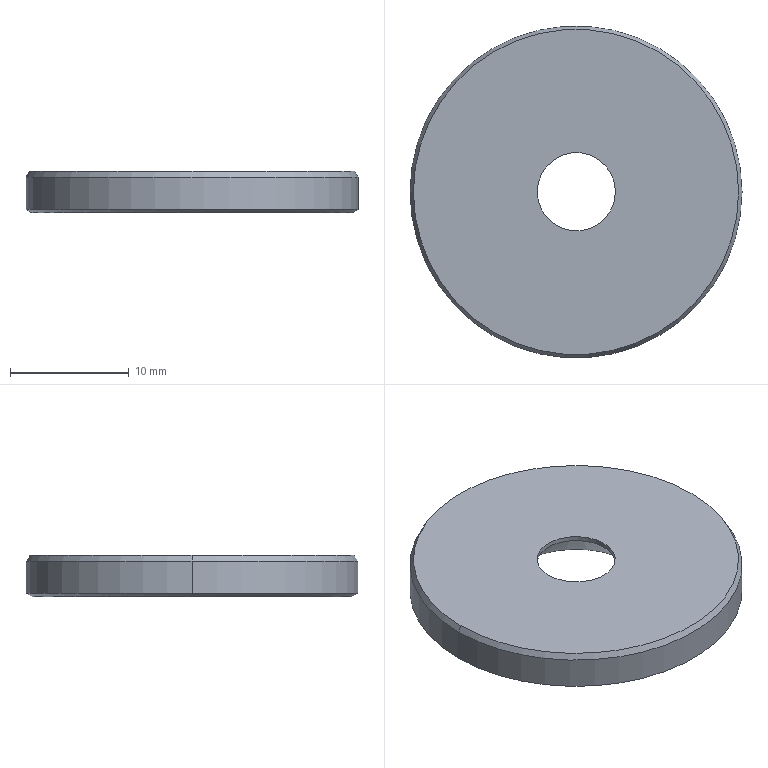Part | SolidWorks | features 3DProfileFeature 1, Chamfer 1, Extrusion 1, HoleWzd 1 | 1 solid | 12 faces | box 28 x 28 x 3.5 mm | volume 1892 mm3 | cone 6 | cylinder 4 | plane 2 | commonest cylinder face diameters 6.6 x2 28 x2
STEP:
#1=CARTESIAN_POINT('',(3.329,0.01727,3.1));
#2=VERTEX_POINT('',#1);
#3=CARTESIAN_POINT('',(-3.271,0.01727,3.1));
#4=VERTEX_POINT('',#3);
#5=CARTESIAN_POINT('',(0.02853,0.01727,3.1));
#6=DIRECTION('',(0.,0.,-1.));
#7=DIRECTION('',(-1.,0.,0.));
#8=AXIS2_PLACEMENT_3D('',#5,#6,#7);
#9=CIRCLE('',#8,3.3);
#10=EDGE_CURVE('',#2,#4,#9,.T.);
#11=ORIENTED_EDGE('',*,*,#10,.F.);
#12=CARTESIAN_POINT('',(6.429,0.01727,0.));
#13=VERTEX_POINT('',#12);
#14=CARTESIAN_POINT('',(6.429,0.01727,0.));
#15=DIRECTION('',(0.7071,0.,-0.7071));
#16=VECTOR('',#15,1000.);
#17=LINE('',#14,#16);
#18=EDGE_CURVE('',#2,#13,#17,.T.);
#19=ORIENTED_EDGE('',*,*,#18,.T.);
#20=CARTESIAN_POINT('',(-6.371,0.01727,0.));
#21=VERTEX_POINT('',#20);
#22=CARTESIAN_POINT('',(0.02853,0.01727,0.));
#23=DIRECTION('',(0.,0.,-1.));
#24=DIRECTION('',(-1.,0.,0.));
#25=AXIS2_PLACEMENT_3D('',#22,#23,#24);
#26=CIRCLE('',#25,6.4);
#27=EDGE_CURVE('',#13,#21,#26,.T.);
#28=ORIENTED_EDGE('',*,*,#27,.T.);
#29=CARTESIAN_POINT('',(-6.371,0.01727,0.));
#30=DIRECTION('',(-0.7071,0.,-0.7071));
#31=VECTOR('',#30,1000.);
#32=LINE('',#29,#31);
#33=EDGE_CURVE('',#4,#21,#32,.T.);
#34=ORIENTED_EDGE('',*,*,#33,.F.);
#35=EDGE_LOOP('',(#11,#19,#28,#34));
#36=FACE_OUTER_BOUND('',#35,.T.);
#37=CARTESIAN_POINT('',(0.02853,0.01727,0.));
#38=DIRECTION('',(0.,0.,-1.));
#39=DIRECTION('',(-1.,0.,0.));
#40=AXIS2_PLACEMENT_3D('',#37,#38,#39);
#41=CONICAL_SURFACE('',#40,6.4,0.7854);
#42=ADVANCED_FACE('',(#36),#41,.F.);
#43=CARTESIAN_POINT('',(-3.271,0.01727,3.5));
#44=VERTEX_POINT('',#43);
#45=CARTESIAN_POINT('',(3.329,0.01727,3.5));
#46=VERTEX_POINT('',#45);
#47=CARTESIAN_POINT('',(0.02853,0.01727,3.5));
#48=DIRECTION('',(0.,0.,1.));
#49=DIRECTION('',(1.,0.,0.));
#50=AXIS2_PLACEMENT_3D('',#47,#48,#49);
#51=CIRCLE('',#50,3.3);
#52=EDGE_CURVE('',#44,#46,#51,.T.);
#53=ORIENTED_EDGE('',*,*,#52,.T.);
#54=CARTESIAN_POINT('',(3.329,0.01727,0.));
#55=DIRECTION('',(0.,0.,-1.));
#56=VECTOR('',#55,1000.);
#57=LINE('',#54,#56);
#58=EDGE_CURVE('',#46,#2,#57,.T.);
#59=ORIENTED_EDGE('',*,*,#58,.T.);
#60=ORIENTED_EDGE('',*,*,#10,.T.);
#61=CARTESIAN_POINT('',(-3.271,0.01727,0.));
#62=DIRECTION('',(0.,0.,-1.));
#63=VECTOR('',#62,1000.);
#64=LINE('',#61,#63);
#65=EDGE_CURVE('',#44,#4,#64,.T.);
#66=ORIENTED_EDGE('',*,*,#65,.F.);
#67=EDGE_LOOP('',(#53,#59,#60,#66));
#68=FACE_OUTER_BOUND('',#67,.T.);
#69=CARTESIAN_POINT('',(0.02853,0.01727,0.));
#70=DIRECTION('',(0.,0.,-1.));
#71=DIRECTION('',(-1.,0.,0.));
#72=AXIS2_PLACEMENT_3D('',#69,#70,#71);
#73=CYLINDRICAL_SURFACE('',#72,3.3);
#74=ADVANCED_FACE('',(#68),#73,.F.);
#75=CARTESIAN_POINT('',(13.711,0.,3.5));
#76=VERTEX_POINT('',#75);
#77=CARTESIAN_POINT('',(-13.711,0.,3.5));
#78=VERTEX_POINT('',#77);
#79=CARTESIAN_POINT('',(0.,0.,3.5));
#80=DIRECTION('',(0.,0.,1.));
#81=DIRECTION('',(1.,0.,0.));
#82=AXIS2_PLACEMENT_3D('',#79,#80,#81);
#83=CIRCLE('',#82,13.711);
#84=EDGE_CURVE('',#76,#78,#83,.T.);
#85=ORIENTED_EDGE('',*,*,#84,.F.);
#86=CARTESIAN_POINT('',(14.,0.,3.));
#87=VERTEX_POINT('',#86);
#88=CARTESIAN_POINT('',(13.711,0.,3.5));
#89=DIRECTION('',(0.5,0.,-0.866));
#90=VECTOR('',#89,1000.);
#91=LINE('',#88,#90);
#92=EDGE_CURVE('',#76,#87,#91,.T.);
#93=ORIENTED_EDGE('',*,*,#92,.T.);
#94=CARTESIAN_POINT('',(-14.,0.,3.));
#95=VERTEX_POINT('',#94);
#96=CARTESIAN_POINT('',(0.,0.,3.));
#97=DIRECTION('',(0.,0.,-1.));
#98=DIRECTION('',(1.,0.,0.));
#99=AXIS2_PLACEMENT_3D('',#96,#97,#98);
#100=CIRCLE('',#99,14.);
#101=EDGE_CURVE('',#95,#87,#100,.T.);
#102=ORIENTED_EDGE('',*,*,#101,.F.);
#103=CARTESIAN_POINT('',(-13.711,0.,3.5));
#104=DIRECTION('',(-0.5,0.,-0.866));
#105=VECTOR('',#104,1000.);
#106=LINE('',#103,#105);
#107=EDGE_CURVE('',#78,#95,#106,.T.);
#108=ORIENTED_EDGE('',*,*,#107,.F.);
#109=EDGE_LOOP('',(#85,#93,#102,#108));
#110=FACE_OUTER_BOUND('',#109,.T.);
#111=CARTESIAN_POINT('',(0.,0.,3.5));
#112=DIRECTION('',(0.,0.,-1.));
#113=DIRECTION('',(-1.,0.,0.));
#114=AXIS2_PLACEMENT_3D('',#111,#112,#113);
#115=CONICAL_SURFACE('',#114,13.711,0.5236);
#116=ADVANCED_FACE('',(#110),#115,.T.);
#117=CARTESIAN_POINT('',(-13.5,0.,0.));
#118=VERTEX_POINT('',#117);
#119=CARTESIAN_POINT('',(13.5,0.,0.));
#120=VERTEX_POINT('',#119);
#121=CARTESIAN_POINT('',(0.,0.,0.));
#122=DIRECTION('',(0.,0.,-1.));
#123=DIRECTION('',(1.,0.,0.));
#124=AXIS2_PLACEMENT_3D('',#121,#122,#123);
#125=CIRCLE('',#124,13.5);
#126=EDGE_CURVE('',#118,#120,#125,.T.);
#127=ORIENTED_EDGE('',*,*,#126,.F.);
#128=CARTESIAN_POINT('',(-14.,0.,0.2887));
#129=VERTEX_POINT('',#128);
#130=CARTESIAN_POINT('',(-14.,0.,0.2887));
#131=DIRECTION('',(-0.866,0.,0.5));
#132=VECTOR('',#131,1000.);
#133=LINE('',#130,#132);
#134=EDGE_CURVE('',#118,#129,#133,.T.);
#135=ORIENTED_EDGE('',*,*,#134,.T.);
#136=CARTESIAN_POINT('',(14.,0.,0.2887));
#137=VERTEX_POINT('',#136);
#138=CARTESIAN_POINT('',(0.,0.,0.2887));
#139=DIRECTION('',(0.,0.,1.));
#140=DIRECTION('',(1.,0.,0.));
#141=AXIS2_PLACEMENT_3D('',#138,#139,#140);
#142=CIRCLE('',#141,14.);
#143=EDGE_CURVE('',#137,#129,#142,.T.);
#144=ORIENTED_EDGE('',*,*,#143,.F.);
#145=CARTESIAN_POINT('',(14.,0.,0.2887));
#146=DIRECTION('',(0.866,0.,0.5));
#147=VECTOR('',#146,1000.);
#148=LINE('',#145,#147);
#149=EDGE_CURVE('',#120,#137,#148,.T.);
#150=ORIENTED_EDGE('',*,*,#149,.F.);
#151=EDGE_LOOP('',(#127,#135,#144,#150));
#152=FACE_OUTER_BOUND('',#151,.T.);
#153=CARTESIAN_POINT('',(0.,0.,0.2887));
#154=DIRECTION('',(0.,0.,1.));
#155=DIRECTION('',(1.,0.,0.));
#156=AXIS2_PLACEMENT_3D('',#153,#154,#155);
#157=CONICAL_SURFACE('',#156,14.,1.047);
#158=ADVANCED_FACE('',(#152),#157,.T.);
#159=ORIENTED_EDGE('',*,*,#101,.T.);
#160=CARTESIAN_POINT('',(14.,0.,3.5));
#161=DIRECTION('',(0.,0.,-1.));
#162=VECTOR('',#161,1000.);
#163=LINE('',#160,#162);
#164=EDGE_CURVE('',#87,#137,#163,.T.);
#165=ORIENTED_EDGE('',*,*,#164,.T.);
#166=ORIENTED_EDGE('',*,*,#143,.T.);
#167=CARTESIAN_POINT('',(-14.,0.,3.5));
#168=DIRECTION('',(0.,0.,-1.));
#169=VECTOR('',#168,1000.);
#170=LINE('',#167,#169);
#171=EDGE_CURVE('',#95,#129,#170,.T.);
#172=ORIENTED_EDGE('',*,*,#171,.F.);
#173=EDGE_LOOP('',(#159,#165,#166,#172));
#174=FACE_OUTER_BOUND('',#173,.T.);
#175=CARTESIAN_POINT('',(0.,0.,3.5));
#176=DIRECTION('',(0.,0.,-1.));
#177=DIRECTION('',(-1.,0.,0.));
#178=AXIS2_PLACEMENT_3D('',#175,#176,#177);
#179=CYLINDRICAL_SURFACE('',#178,14.);
#180=ADVANCED_FACE('',(#174),#179,.T.);
#181=ORIENTED_EDGE('',*,*,#164,.F.);
#182=CARTESIAN_POINT('',(0.,0.,3.));
#183=DIRECTION('',(0.,0.,-1.));
#184=DIRECTION('',(1.,0.,0.));
#185=AXIS2_PLACEMENT_3D('',#182,#183,#184);
#186=CIRCLE('',#185,14.);
#187=EDGE_CURVE('',#87,#95,#186,.T.);
#188=ORIENTED_EDGE('',*,*,#187,.T.);
#189=ORIENTED_EDGE('',*,*,#171,.T.);
#190=CARTESIAN_POINT('',(0.,0.,0.2887));
#191=DIRECTION('',(0.,0.,1.));
#192=DIRECTION('',(1.,0.,0.));
#193=AXIS2_PLACEMENT_3D('',#190,#191,#192);
#194=CIRCLE('',#193,14.);
#195=EDGE_CURVE('',#129,#137,#194,.T.);
#196=ORIENTED_EDGE('',*,*,#195,.T.);
#197=EDGE_LOOP('',(#181,#188,#189,#196));
#198=FACE_OUTER_BOUND('',#197,.T.);
#199=CARTESIAN_POINT('',(0.,0.,3.5));
#200=DIRECTION('',(0.,0.,-1.));
#201=DIRECTION('',(-1.,0.,0.));
#202=AXIS2_PLACEMENT_3D('',#199,#200,#201);
#203=CYLINDRICAL_SURFACE('',#202,14.);
#204=ADVANCED_FACE('',(#198),#203,.T.);
#205=ORIENTED_EDGE('',*,*,#52,.F.);
#206=CARTESIAN_POINT('',(0.02853,0.01727,3.5));
#207=DIRECTION('',(0.,0.,1.));
#208=DIRECTION('',(1.,0.,0.));
#209=AXIS2_PLACEMENT_3D('',#206,#207,#208);
#210=CIRCLE('',#209,3.3);
#211=EDGE_CURVE('',#46,#44,#210,.T.);
#212=ORIENTED_EDGE('',*,*,#211,.F.);
#213=EDGE_LOOP('',(#205,#212));
#214=FACE_BOUND('',#213,.T.);
#215=CARTESIAN_POINT('',(0.,0.,3.5));
#216=DIRECTION('',(0.,0.,1.));
#217=DIRECTION('',(1.,0.,0.));
#218=AXIS2_PLACEMENT_3D('',#215,#216,#217);
#219=CIRCLE('',#218,13.711);
#220=EDGE_CURVE('',#78,#76,#219,.T.);
#221=ORIENTED_EDGE('',*,*,#220,.T.);
#222=ORIENTED_EDGE('',*,*,#84,.T.);
#223=EDGE_LOOP('',(#221,#222));
#224=FACE_OUTER_BOUND('',#223,.T.);
#225=CARTESIAN_POINT('',(0.,0.,3.5));
#226=DIRECTION('',(0.,0.,1.));
#227=DIRECTION('',(1.,0.,0.));
#228=AXIS2_PLACEMENT_3D('',#225,#226,#227);
#229=PLANE('',#228);
#230=ADVANCED_FACE('',(#214,#224),#229,.T.);
#231=CARTESIAN_POINT('',(0.02853,0.01727,0.));
#232=DIRECTION('',(0.,0.,-1.));
#233=DIRECTION('',(-1.,0.,0.));
#234=AXIS2_PLACEMENT_3D('',#231,#232,#233);
#235=CIRCLE('',#234,6.4);
#236=EDGE_CURVE('',#21,#13,#235,.T.);
#237=ORIENTED_EDGE('',*,*,#236,.F.);
#238=ORIENTED_EDGE('',*,*,#27,.F.);
#239=EDGE_LOOP('',(#237,#238));
#240=FACE_BOUND('',#239,.T.);
#241=CARTESIAN_POINT('',(0.,0.,0.));
#242=DIRECTION('',(0.,0.,-1.));
#243=DIRECTION('',(1.,0.,0.));
#244=AXIS2_PLACEMENT_3D('',#241,#242,#243);
#245=CIRCLE('',#244,13.5);
#246=EDGE_CURVE('',#120,#118,#245,.T.);
#247=ORIENTED_EDGE('',*,*,#246,.T.);
#248=ORIENTED_EDGE('',*,*,#126,.T.);
#249=EDGE_LOOP('',(#247,#248));
#250=FACE_OUTER_BOUND('',#249,.T.);
#251=CARTESIAN_POINT('',(0.,0.,0.));
#252=DIRECTION('',(0.,0.,1.));
#253=DIRECTION('',(1.,0.,0.));
#254=AXIS2_PLACEMENT_3D('',#251,#252,#253);
#255=PLANE('',#254);
#256=ADVANCED_FACE('',(#240,#250),#255,.F.);
#257=ORIENTED_EDGE('',*,*,#134,.F.);
#258=ORIENTED_EDGE('',*,*,#246,.F.);
#259=ORIENTED_EDGE('',*,*,#149,.T.);
#260=ORIENTED_EDGE('',*,*,#195,.F.);
#261=EDGE_LOOP('',(#257,#258,#259,#260));
#262=FACE_OUTER_BOUND('',#261,.T.);
#263=CARTESIAN_POINT('',(0.,0.,0.2887));
#264=DIRECTION('',(0.,0.,1.));
#265=DIRECTION('',(1.,0.,0.));
#266=AXIS2_PLACEMENT_3D('',#263,#264,#265);
#267=CONICAL_SURFACE('',#266,14.,1.047);
#268=ADVANCED_FACE('',(#262),#267,.T.);
#269=ORIENTED_EDGE('',*,*,#92,.F.);
#270=ORIENTED_EDGE('',*,*,#220,.F.);
#271=ORIENTED_EDGE('',*,*,#107,.T.);
#272=ORIENTED_EDGE('',*,*,#187,.F.);
#273=EDGE_LOOP('',(#269,#270,#271,#272));
#274=FACE_OUTER_BOUND('',#273,.T.);
#275=CARTESIAN_POINT('',(0.,0.,3.5));
#276=DIRECTION('',(0.,0.,-1.));
#277=DIRECTION('',(-1.,0.,0.));
#278=AXIS2_PLACEMENT_3D('',#275,#276,#277);
#279=CONICAL_SURFACE('',#278,13.711,0.5236);
#280=ADVANCED_FACE('',(#274),#279,.T.);
#281=ORIENTED_EDGE('',*,*,#58,.F.);
#282=ORIENTED_EDGE('',*,*,#211,.T.);
#283=ORIENTED_EDGE('',*,*,#65,.T.);
#284=CARTESIAN_POINT('',(0.02853,0.01727,3.1));
#285=DIRECTION('',(0.,0.,-1.));
#286=DIRECTION('',(-1.,0.,0.));
#287=AXIS2_PLACEMENT_3D('',#284,#285,#286);
#288=CIRCLE('',#287,3.3);
#289=EDGE_CURVE('',#4,#2,#288,.T.);
#290=ORIENTED_EDGE('',*,*,#289,.T.);
#291=EDGE_LOOP('',(#281,#282,#283,#290));
#292=FACE_OUTER_BOUND('',#291,.T.);
#293=CARTESIAN_POINT('',(0.02853,0.01727,0.));
#294=DIRECTION('',(0.,0.,-1.));
#295=DIRECTION('',(-1.,0.,0.));
#296=AXIS2_PLACEMENT_3D('',#293,#294,#295);
#297=CYLINDRICAL_SURFACE('',#296,3.3);
#298=ADVANCED_FACE('',(#292),#297,.F.);
#299=ORIENTED_EDGE('',*,*,#18,.F.);
#300=ORIENTED_EDGE('',*,*,#289,.F.);
#301=ORIENTED_EDGE('',*,*,#33,.T.);
#302=ORIENTED_EDGE('',*,*,#236,.T.);
#303=EDGE_LOOP('',(#299,#300,#301,#302));
#304=FACE_OUTER_BOUND('',#303,.T.);
#305=CARTESIAN_POINT('',(0.02853,0.01727,0.));
#306=DIRECTION('',(0.,0.,-1.));
#307=DIRECTION('',(-1.,0.,0.));
#308=AXIS2_PLACEMENT_3D('',#305,#306,#307);
#309=CONICAL_SURFACE('',#308,6.4,0.7854);
#310=ADVANCED_FACE('',(#304),#309,.F.);
#311=CLOSED_SHELL('',(#42,#74,#116,#158,#180,#204,#230,#256,#268,#280,#298,#310));
#312=MANIFOLD_SOLID_BREP('',#311);
#313=CARTESIAN_POINT('',(0.,0.,0.));
#314=DIRECTION('',(0.,0.,1.));
#315=DIRECTION('',(1.,0.,0.));
#316=AXIS2_PLACEMENT_3D('',#313,#314,#315);
#317=(LENGTH_UNIT()NAMED_UNIT(*)SI_UNIT(.MILLI.,.METRE.));
#318=UNCERTAINTY_MEASURE_WITH_UNIT(LENGTH_MEASURE(0.00001),#317,'','');
#319=(NAMED_UNIT(*)PLANE_ANGLE_UNIT()SI_UNIT($,.RADIAN.));
#320=(NAMED_UNIT(*)SI_UNIT($,.STERADIAN.)SOLID_ANGLE_UNIT());
#321=(GEOMETRIC_REPRESENTATION_CONTEXT(3)GLOBAL_UNCERTAINTY_ASSIGNED_CONTEXT((#318))GLOBAL_UNIT_ASSIGNED_CONTEXT((#317,#319,#320))REPRESENTATION_CONTEXT('',''));
#322=ADVANCED_BREP_SHAPE_REPRESENTATION('',(#312,#316),#321);